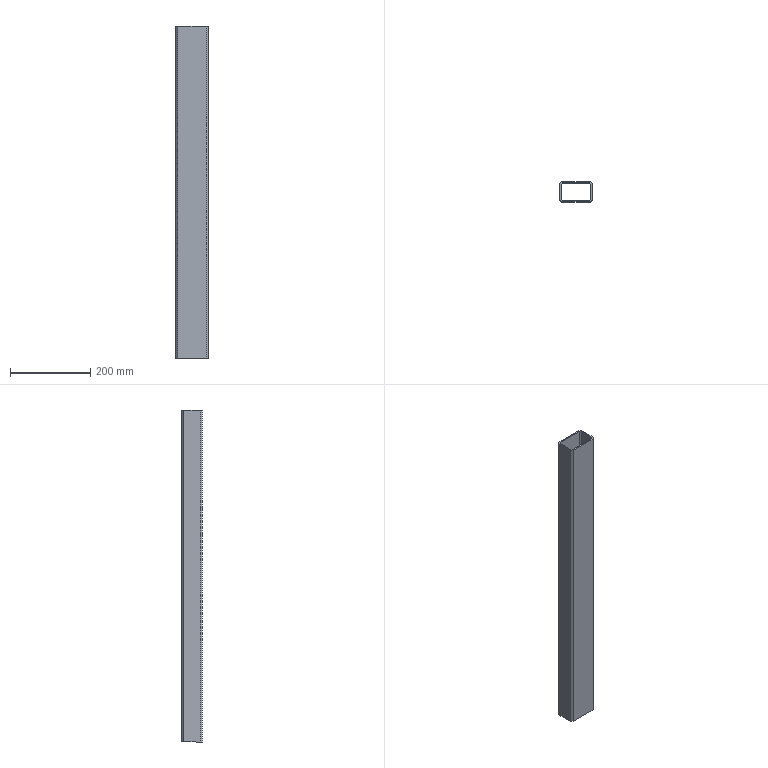Part | SolidWorks | features BaseBody 1 | 1 solid | 18 faces | box 80 x 50 x 825 mm | volume 589899 mm3 | plane 18
STEP:
#1=CARTESIAN_POINT('',(43.047,1567.079,-399.));
#2=VERTEX_POINT('',#1);
#3=CARTESIAN_POINT('',(113.047,1567.079,-399.));
#4=VERTEX_POINT('',#3);
#5=CARTESIAN_POINT('',(38.047,1567.079,-399.));
#6=DIRECTION('',(1.,0.,0.));
#7=VECTOR('',#6,1000.);
#8=LINE('',#5,#7);
#9=EDGE_CURVE('',#2,#4,#8,.T.);
#10=ORIENTED_EDGE('',*,*,#9,.F.);
#11=CARTESIAN_POINT('',(43.047,1567.079,-1224.));
#12=VERTEX_POINT('',#11);
#13=CARTESIAN_POINT('',(43.047,1567.079,-449.));
#14=DIRECTION('',(0.,0.,1.));
#15=VECTOR('',#14,1000.);
#16=LINE('',#13,#15);
#17=EDGE_CURVE('',#12,#2,#16,.T.);
#18=ORIENTED_EDGE('',*,*,#17,.F.);
#19=CARTESIAN_POINT('',(113.047,1567.079,-1224.));
#20=VERTEX_POINT('',#19);
#21=CARTESIAN_POINT('',(38.047,1567.079,-1224.));
#22=DIRECTION('',(-1.,0.,0.));
#23=VECTOR('',#22,1000.);
#24=LINE('',#21,#23);
#25=EDGE_CURVE('',#20,#12,#24,.T.);
#26=ORIENTED_EDGE('',*,*,#25,.F.);
#27=CARTESIAN_POINT('',(113.047,1567.079,-449.));
#28=DIRECTION('',(0.,0.,-1.));
#29=VECTOR('',#28,1000.);
#30=LINE('',#27,#29);
#31=EDGE_CURVE('',#4,#20,#30,.T.);
#32=ORIENTED_EDGE('',*,*,#31,.F.);
#33=EDGE_LOOP('',(#10,#18,#26,#32));
#34=FACE_OUTER_BOUND('',#33,.T.);
#35=CARTESIAN_POINT('',(38.047,1567.079,-449.));
#36=DIRECTION('',(0.,1.,0.));
#37=DIRECTION('',(0.,0.,1.));
#38=AXIS2_PLACEMENT_3D('',#35,#36,#37);
#39=PLANE('',#38);
#40=ADVANCED_FACE('',(#34),#39,.F.);
#41=CARTESIAN_POINT('',(118.047,1572.079,-1224.));
#42=VERTEX_POINT('',#41);
#43=CARTESIAN_POINT('',(118.047,1572.079,-1224.));
#44=DIRECTION('',(-0.7071,-0.7071,0.));
#45=VECTOR('',#44,1000.);
#46=LINE('',#43,#45);
#47=EDGE_CURVE('',#42,#20,#46,.T.);
#48=ORIENTED_EDGE('',*,*,#47,.F.);
#49=CARTESIAN_POINT('',(118.047,1572.079,-399.));
#50=VERTEX_POINT('',#49);
#51=CARTESIAN_POINT('',(118.047,1572.079,-449.));
#52=DIRECTION('',(0.,0.,-1.));
#53=VECTOR('',#52,1000.);
#54=LINE('',#51,#53);
#55=EDGE_CURVE('',#50,#42,#54,.T.);
#56=ORIENTED_EDGE('',*,*,#55,.F.);
#57=CARTESIAN_POINT('',(118.047,1572.079,-399.));
#58=DIRECTION('',(0.7071,0.7071,0.));
#59=VECTOR('',#58,1000.);
#60=LINE('',#57,#59);
#61=EDGE_CURVE('',#4,#50,#60,.T.);
#62=ORIENTED_EDGE('',*,*,#61,.F.);
#63=ORIENTED_EDGE('',*,*,#31,.T.);
#64=EDGE_LOOP('',(#48,#56,#62,#63));
#65=FACE_OUTER_BOUND('',#64,.T.);
#66=CARTESIAN_POINT('',(118.047,1572.079,-449.));
#67=DIRECTION('',(-0.7071,0.7071,0.));
#68=DIRECTION('',(-0.7071,-0.7071,0.));
#69=AXIS2_PLACEMENT_3D('',#66,#67,#68);
#70=PLANE('',#69);
#71=ADVANCED_FACE('',(#65),#70,.F.);
#72=CARTESIAN_POINT('',(115.047,1573.321,-399.));
#73=VERTEX_POINT('',#72);
#74=CARTESIAN_POINT('',(111.804,1570.079,-399.));
#75=VERTEX_POINT('',#74);
#76=CARTESIAN_POINT('',(115.047,1573.321,-399.));
#77=DIRECTION('',(-0.7071,-0.7071,0.));
#78=VECTOR('',#77,1000.);
#79=LINE('',#76,#78);
#80=EDGE_CURVE('',#73,#75,#79,.T.);
#81=ORIENTED_EDGE('',*,*,#80,.T.);
#82=CARTESIAN_POINT('',(44.289,1570.079,-399.));
#83=VERTEX_POINT('',#82);
#84=CARTESIAN_POINT('',(118.047,1570.079,-399.));
#85=DIRECTION('',(-1.,0.,0.));
#86=VECTOR('',#85,1000.);
#87=LINE('',#84,#86);
#88=EDGE_CURVE('',#75,#83,#87,.T.);
#89=ORIENTED_EDGE('',*,*,#88,.T.);
#90=CARTESIAN_POINT('',(41.047,1573.321,-399.));
#91=VERTEX_POINT('',#90);
#92=CARTESIAN_POINT('',(44.289,1570.079,-399.));
#93=DIRECTION('',(-0.7071,0.7071,0.));
#94=VECTOR('',#93,1000.);
#95=LINE('',#92,#94);
#96=EDGE_CURVE('',#83,#91,#95,.T.);
#97=ORIENTED_EDGE('',*,*,#96,.T.);
#98=CARTESIAN_POINT('',(41.047,1610.836,-399.));
#99=VERTEX_POINT('',#98);
#100=CARTESIAN_POINT('',(41.047,1567.079,-399.));
#101=DIRECTION('',(0.,1.,0.));
#102=VECTOR('',#101,1000.);
#103=LINE('',#100,#102);
#104=EDGE_CURVE('',#91,#99,#103,.T.);
#105=ORIENTED_EDGE('',*,*,#104,.T.);
#106=CARTESIAN_POINT('',(44.289,1614.079,-399.));
#107=VERTEX_POINT('',#106);
#108=CARTESIAN_POINT('',(41.047,1610.836,-399.));
#109=DIRECTION('',(0.7071,0.7071,0.));
#110=VECTOR('',#109,1000.);
#111=LINE('',#108,#110);
#112=EDGE_CURVE('',#99,#107,#111,.T.);
#113=ORIENTED_EDGE('',*,*,#112,.T.);
#114=CARTESIAN_POINT('',(111.804,1614.079,-399.));
#115=VERTEX_POINT('',#114);
#116=CARTESIAN_POINT('',(118.047,1614.079,-399.));
#117=DIRECTION('',(1.,0.,0.));
#118=VECTOR('',#117,1000.);
#119=LINE('',#116,#118);
#120=EDGE_CURVE('',#107,#115,#119,.T.);
#121=ORIENTED_EDGE('',*,*,#120,.T.);
#122=CARTESIAN_POINT('',(115.047,1610.836,-399.));
#123=VERTEX_POINT('',#122);
#124=CARTESIAN_POINT('',(111.804,1614.079,-399.));
#125=DIRECTION('',(0.7071,-0.7071,0.));
#126=VECTOR('',#125,1000.);
#127=LINE('',#124,#126);
#128=EDGE_CURVE('',#115,#123,#127,.T.);
#129=ORIENTED_EDGE('',*,*,#128,.T.);
#130=CARTESIAN_POINT('',(115.047,1567.079,-399.));
#131=DIRECTION('',(0.,-1.,0.));
#132=VECTOR('',#131,1000.);
#133=LINE('',#130,#132);
#134=EDGE_CURVE('',#123,#73,#133,.T.);
#135=ORIENTED_EDGE('',*,*,#134,.T.);
#136=EDGE_LOOP('',(#81,#89,#97,#105,#113,#121,#129,#135));
#137=FACE_BOUND('',#136,.T.);
#138=CARTESIAN_POINT('',(38.047,1572.079,-399.));
#139=VERTEX_POINT('',#138);
#140=CARTESIAN_POINT('',(38.047,1572.079,-399.));
#141=DIRECTION('',(0.7071,-0.7071,0.));
#142=VECTOR('',#141,1000.);
#143=LINE('',#140,#142);
#144=EDGE_CURVE('',#139,#2,#143,.T.);
#145=ORIENTED_EDGE('',*,*,#144,.T.);
#146=ORIENTED_EDGE('',*,*,#9,.T.);
#147=ORIENTED_EDGE('',*,*,#61,.T.);
#148=CARTESIAN_POINT('',(118.047,1612.079,-399.));
#149=VERTEX_POINT('',#148);
#150=CARTESIAN_POINT('',(118.047,1567.079,-399.));
#151=DIRECTION('',(0.,1.,0.));
#152=VECTOR('',#151,1000.);
#153=LINE('',#150,#152);
#154=EDGE_CURVE('',#50,#149,#153,.T.);
#155=ORIENTED_EDGE('',*,*,#154,.T.);
#156=CARTESIAN_POINT('',(113.047,1617.079,-399.));
#157=VERTEX_POINT('',#156);
#158=CARTESIAN_POINT('',(118.047,1612.079,-399.));
#159=DIRECTION('',(-0.7071,0.7071,0.));
#160=VECTOR('',#159,1000.);
#161=LINE('',#158,#160);
#162=EDGE_CURVE('',#149,#157,#161,.T.);
#163=ORIENTED_EDGE('',*,*,#162,.T.);
#164=CARTESIAN_POINT('',(43.047,1617.079,-399.));
#165=VERTEX_POINT('',#164);
#166=CARTESIAN_POINT('',(118.047,1617.079,-399.));
#167=DIRECTION('',(-1.,0.,0.));
#168=VECTOR('',#167,1000.);
#169=LINE('',#166,#168);
#170=EDGE_CURVE('',#157,#165,#169,.T.);
#171=ORIENTED_EDGE('',*,*,#170,.T.);
#172=CARTESIAN_POINT('',(38.047,1612.079,-399.));
#173=VERTEX_POINT('',#172);
#174=CARTESIAN_POINT('',(43.047,1617.079,-399.));
#175=DIRECTION('',(-0.7071,-0.7071,0.));
#176=VECTOR('',#175,1000.);
#177=LINE('',#174,#176);
#178=EDGE_CURVE('',#165,#173,#177,.T.);
#179=ORIENTED_EDGE('',*,*,#178,.T.);
#180=CARTESIAN_POINT('',(38.047,1567.079,-399.));
#181=DIRECTION('',(0.,-1.,0.));
#182=VECTOR('',#181,1000.);
#183=LINE('',#180,#182);
#184=EDGE_CURVE('',#173,#139,#183,.T.);
#185=ORIENTED_EDGE('',*,*,#184,.T.);
#186=EDGE_LOOP('',(#145,#146,#147,#155,#163,#171,#179,#185));
#187=FACE_OUTER_BOUND('',#186,.T.);
#188=CARTESIAN_POINT('',(118.047,1567.079,-399.));
#189=DIRECTION('',(0.,0.,1.));
#190=DIRECTION('',(1.,0.,0.));
#191=AXIS2_PLACEMENT_3D('',#188,#189,#190);
#192=PLANE('',#191);
#193=ADVANCED_FACE('',(#137,#187),#192,.T.);
#194=CARTESIAN_POINT('',(38.047,1572.079,-1224.));
#195=VERTEX_POINT('',#194);
#196=CARTESIAN_POINT('',(43.047,1567.079,-1224.));
#197=DIRECTION('',(-0.7071,0.7071,0.));
#198=VECTOR('',#197,1000.);
#199=LINE('',#196,#198);
#200=EDGE_CURVE('',#12,#195,#199,.T.);
#201=ORIENTED_EDGE('',*,*,#200,.F.);
#202=ORIENTED_EDGE('',*,*,#17,.T.);
#203=ORIENTED_EDGE('',*,*,#144,.F.);
#204=CARTESIAN_POINT('',(38.047,1572.079,-449.));
#205=DIRECTION('',(0.,0.,1.));
#206=VECTOR('',#205,1000.);
#207=LINE('',#204,#206);
#208=EDGE_CURVE('',#195,#139,#207,.T.);
#209=ORIENTED_EDGE('',*,*,#208,.F.);
#210=EDGE_LOOP('',(#201,#202,#203,#209));
#211=FACE_OUTER_BOUND('',#210,.T.);
#212=CARTESIAN_POINT('',(43.047,1567.079,-449.));
#213=DIRECTION('',(0.7071,0.7071,0.));
#214=DIRECTION('',(-0.7071,0.7071,0.));
#215=AXIS2_PLACEMENT_3D('',#212,#213,#214);
#216=PLANE('',#215);
#217=ADVANCED_FACE('',(#211),#216,.F.);
#218=CARTESIAN_POINT('',(111.804,1614.079,-1224.));
#219=VERTEX_POINT('',#218);
#220=CARTESIAN_POINT('',(115.047,1610.836,-1224.));
#221=VERTEX_POINT('',#220);
#222=CARTESIAN_POINT('',(111.804,1614.079,-1224.));
#223=DIRECTION('',(0.7071,-0.7071,0.));
#224=VECTOR('',#223,1000.);
#225=LINE('',#222,#224);
#226=EDGE_CURVE('',#219,#221,#225,.T.);
#227=ORIENTED_EDGE('',*,*,#226,.F.);
#228=CARTESIAN_POINT('',(44.289,1614.079,-1224.));
#229=VERTEX_POINT('',#228);
#230=CARTESIAN_POINT('',(118.047,1614.079,-1224.));
#231=DIRECTION('',(1.,0.,0.));
#232=VECTOR('',#231,1000.);
#233=LINE('',#230,#232);
#234=EDGE_CURVE('',#229,#219,#233,.T.);
#235=ORIENTED_EDGE('',*,*,#234,.F.);
#236=CARTESIAN_POINT('',(41.047,1610.836,-1224.));
#237=VERTEX_POINT('',#236);
#238=CARTESIAN_POINT('',(41.047,1610.836,-1224.));
#239=DIRECTION('',(0.7071,0.7071,0.));
#240=VECTOR('',#239,1000.);
#241=LINE('',#238,#240);
#242=EDGE_CURVE('',#237,#229,#241,.T.);
#243=ORIENTED_EDGE('',*,*,#242,.F.);
#244=CARTESIAN_POINT('',(41.047,1573.321,-1224.));
#245=VERTEX_POINT('',#244);
#246=CARTESIAN_POINT('',(41.047,1567.079,-1224.));
#247=DIRECTION('',(0.,1.,0.));
#248=VECTOR('',#247,1000.);
#249=LINE('',#246,#248);
#250=EDGE_CURVE('',#245,#237,#249,.T.);
#251=ORIENTED_EDGE('',*,*,#250,.F.);
#252=CARTESIAN_POINT('',(44.289,1570.079,-1224.));
#253=VERTEX_POINT('',#252);
#254=CARTESIAN_POINT('',(44.289,1570.079,-1224.));
#255=DIRECTION('',(-0.7071,0.7071,0.));
#256=VECTOR('',#255,1000.);
#257=LINE('',#254,#256);
#258=EDGE_CURVE('',#253,#245,#257,.T.);
#259=ORIENTED_EDGE('',*,*,#258,.F.);
#260=CARTESIAN_POINT('',(111.804,1570.079,-1224.));
#261=VERTEX_POINT('',#260);
#262=CARTESIAN_POINT('',(118.047,1570.079,-1224.));
#263=DIRECTION('',(-1.,0.,0.));
#264=VECTOR('',#263,1000.);
#265=LINE('',#262,#264);
#266=EDGE_CURVE('',#261,#253,#265,.T.);
#267=ORIENTED_EDGE('',*,*,#266,.F.);
#268=CARTESIAN_POINT('',(115.047,1573.321,-1224.));
#269=VERTEX_POINT('',#268);
#270=CARTESIAN_POINT('',(115.047,1573.321,-1224.));
#271=DIRECTION('',(-0.7071,-0.7071,0.));
#272=VECTOR('',#271,1000.);
#273=LINE('',#270,#272);
#274=EDGE_CURVE('',#269,#261,#273,.T.);
#275=ORIENTED_EDGE('',*,*,#274,.F.);
#276=CARTESIAN_POINT('',(115.047,1567.079,-1224.));
#277=DIRECTION('',(0.,-1.,0.));
#278=VECTOR('',#277,1000.);
#279=LINE('',#276,#278);
#280=EDGE_CURVE('',#221,#269,#279,.T.);
#281=ORIENTED_EDGE('',*,*,#280,.F.);
#282=EDGE_LOOP('',(#227,#235,#243,#251,#259,#267,#275,#281));
#283=FACE_BOUND('',#282,.T.);
#284=ORIENTED_EDGE('',*,*,#25,.T.);
#285=ORIENTED_EDGE('',*,*,#200,.T.);
#286=CARTESIAN_POINT('',(38.047,1612.079,-1224.));
#287=VERTEX_POINT('',#286);
#288=CARTESIAN_POINT('',(38.047,1567.079,-1224.));
#289=DIRECTION('',(0.,-1.,0.));
#290=VECTOR('',#289,1000.);
#291=LINE('',#288,#290);
#292=EDGE_CURVE('',#287,#195,#291,.T.);
#293=ORIENTED_EDGE('',*,*,#292,.F.);
#294=CARTESIAN_POINT('',(43.047,1617.079,-1224.));
#295=VERTEX_POINT('',#294);
#296=CARTESIAN_POINT('',(43.047,1617.079,-1224.));
#297=DIRECTION('',(-0.7071,-0.7071,0.));
#298=VECTOR('',#297,1000.);
#299=LINE('',#296,#298);
#300=EDGE_CURVE('',#295,#287,#299,.T.);
#301=ORIENTED_EDGE('',*,*,#300,.F.);
#302=CARTESIAN_POINT('',(113.047,1617.079,-1224.));
#303=VERTEX_POINT('',#302);
#304=CARTESIAN_POINT('',(118.047,1617.079,-1224.));
#305=DIRECTION('',(-1.,0.,0.));
#306=VECTOR('',#305,1000.);
#307=LINE('',#304,#306);
#308=EDGE_CURVE('',#303,#295,#307,.T.);
#309=ORIENTED_EDGE('',*,*,#308,.F.);
#310=CARTESIAN_POINT('',(118.047,1612.079,-1224.));
#311=VERTEX_POINT('',#310);
#312=CARTESIAN_POINT('',(118.047,1612.079,-1224.));
#313=DIRECTION('',(-0.7071,0.7071,0.));
#314=VECTOR('',#313,1000.);
#315=LINE('',#312,#314);
#316=EDGE_CURVE('',#311,#303,#315,.T.);
#317=ORIENTED_EDGE('',*,*,#316,.F.);
#318=CARTESIAN_POINT('',(118.047,1567.079,-1224.));
#319=DIRECTION('',(0.,1.,0.));
#320=VECTOR('',#319,1000.);
#321=LINE('',#318,#320);
#322=EDGE_CURVE('',#42,#311,#321,.T.);
#323=ORIENTED_EDGE('',*,*,#322,.F.);
#324=ORIENTED_EDGE('',*,*,#47,.T.);
#325=EDGE_LOOP('',(#284,#285,#293,#301,#309,#317,#323,#324));
#326=FACE_OUTER_BOUND('',#325,.T.);
#327=CARTESIAN_POINT('',(118.047,1567.079,-1224.));
#328=DIRECTION('',(0.,0.,1.));
#329=DIRECTION('',(1.,0.,0.));
#330=AXIS2_PLACEMENT_3D('',#327,#328,#329);
#331=PLANE('',#330);
#332=ADVANCED_FACE('',(#283,#326),#331,.F.);
#333=ORIENTED_EDGE('',*,*,#322,.T.);
#334=CARTESIAN_POINT('',(118.047,1612.079,-449.));
#335=DIRECTION('',(0.,0.,-1.));
#336=VECTOR('',#335,1000.);
#337=LINE('',#334,#336);
#338=EDGE_CURVE('',#149,#311,#337,.T.);
#339=ORIENTED_EDGE('',*,*,#338,.F.);
#340=ORIENTED_EDGE('',*,*,#154,.F.);
#341=ORIENTED_EDGE('',*,*,#55,.T.);
#342=EDGE_LOOP('',(#333,#339,#340,#341));
#343=FACE_OUTER_BOUND('',#342,.T.);
#344=CARTESIAN_POINT('',(118.047,1567.079,-449.));
#345=DIRECTION('',(-1.,0.,0.));
#346=DIRECTION('',(0.,0.,1.));
#347=AXIS2_PLACEMENT_3D('',#344,#345,#346);
#348=PLANE('',#347);
#349=ADVANCED_FACE('',(#343),#348,.F.);
#350=CARTESIAN_POINT('',(111.804,1570.079,-449.));
#351=DIRECTION('',(0.,0.,-1.));
#352=VECTOR('',#351,1000.);
#353=LINE('',#350,#352);
#354=EDGE_CURVE('',#75,#261,#353,.T.);
#355=ORIENTED_EDGE('',*,*,#354,.T.);
#356=ORIENTED_EDGE('',*,*,#266,.T.);
#357=CARTESIAN_POINT('',(44.289,1570.079,-449.));
#358=DIRECTION('',(0.,0.,1.));
#359=VECTOR('',#358,1000.);
#360=LINE('',#357,#359);
#361=EDGE_CURVE('',#253,#83,#360,.T.);
#362=ORIENTED_EDGE('',*,*,#361,.T.);
#363=ORIENTED_EDGE('',*,*,#88,.F.);
#364=EDGE_LOOP('',(#355,#356,#362,#363));
#365=FACE_OUTER_BOUND('',#364,.T.);
#366=CARTESIAN_POINT('',(38.047,1570.079,-449.));
#367=DIRECTION('',(0.,1.,0.));
#368=DIRECTION('',(0.,0.,1.));
#369=AXIS2_PLACEMENT_3D('',#366,#367,#368);
#370=PLANE('',#369);
#371=ADVANCED_FACE('',(#365),#370,.T.);
#372=ORIENTED_EDGE('',*,*,#354,.F.);
#373=ORIENTED_EDGE('',*,*,#80,.F.);
#374=CARTESIAN_POINT('',(115.047,1573.321,-449.));
#375=DIRECTION('',(0.,0.,-1.));
#376=VECTOR('',#375,1000.);
#377=LINE('',#374,#376);
#378=EDGE_CURVE('',#73,#269,#377,.T.);
#379=ORIENTED_EDGE('',*,*,#378,.T.);
#380=ORIENTED_EDGE('',*,*,#274,.T.);
#381=EDGE_LOOP('',(#372,#373,#379,#380));
#382=FACE_OUTER_BOUND('',#381,.T.);
#383=CARTESIAN_POINT('',(115.925,1574.2,-449.));
#384=DIRECTION('',(-0.7071,0.7071,0.));
#385=DIRECTION('',(-0.7071,-0.7071,0.));
#386=AXIS2_PLACEMENT_3D('',#383,#384,#385);
#387=PLANE('',#386);
#388=ADVANCED_FACE('',(#382),#387,.T.);
#389=ORIENTED_EDGE('',*,*,#378,.F.);
#390=ORIENTED_EDGE('',*,*,#134,.F.);
#391=CARTESIAN_POINT('',(115.047,1610.836,-449.));
#392=DIRECTION('',(0.,0.,-1.));
#393=VECTOR('',#392,1000.);
#394=LINE('',#391,#393);
#395=EDGE_CURVE('',#123,#221,#394,.T.);
#396=ORIENTED_EDGE('',*,*,#395,.T.);
#397=ORIENTED_EDGE('',*,*,#280,.T.);
#398=EDGE_LOOP('',(#389,#390,#396,#397));
#399=FACE_OUTER_BOUND('',#398,.T.);
#400=CARTESIAN_POINT('',(115.047,1567.079,-449.));
#401=DIRECTION('',(-1.,0.,0.));
#402=DIRECTION('',(0.,0.,1.));
#403=AXIS2_PLACEMENT_3D('',#400,#401,#402);
#404=PLANE('',#403);
#405=ADVANCED_FACE('',(#399),#404,.T.);
#406=ORIENTED_EDGE('',*,*,#395,.F.);
#407=ORIENTED_EDGE('',*,*,#128,.F.);
#408=CARTESIAN_POINT('',(111.804,1614.079,-449.));
#409=DIRECTION('',(0.,0.,-1.));
#410=VECTOR('',#409,1000.);
#411=LINE('',#408,#410);
#412=EDGE_CURVE('',#115,#219,#411,.T.);
#413=ORIENTED_EDGE('',*,*,#412,.T.);
#414=ORIENTED_EDGE('',*,*,#226,.T.);
#415=EDGE_LOOP('',(#406,#407,#413,#414));
#416=FACE_OUTER_BOUND('',#415,.T.);
#417=CARTESIAN_POINT('',(110.925,1614.957,-449.));
#418=DIRECTION('',(-0.7071,-0.7071,0.));
#419=DIRECTION('',(0.7071,-0.7071,0.));
#420=AXIS2_PLACEMENT_3D('',#417,#418,#419);
#421=PLANE('',#420);
#422=ADVANCED_FACE('',(#416),#421,.T.);
#423=ORIENTED_EDGE('',*,*,#412,.F.);
#424=ORIENTED_EDGE('',*,*,#120,.F.);
#425=CARTESIAN_POINT('',(44.289,1614.079,-449.));
#426=DIRECTION('',(0.,0.,-1.));
#427=VECTOR('',#426,1000.);
#428=LINE('',#425,#427);
#429=EDGE_CURVE('',#107,#229,#428,.T.);
#430=ORIENTED_EDGE('',*,*,#429,.T.);
#431=ORIENTED_EDGE('',*,*,#234,.T.);
#432=EDGE_LOOP('',(#423,#424,#430,#431));
#433=FACE_OUTER_BOUND('',#432,.T.);
#434=CARTESIAN_POINT('',(38.047,1614.079,-449.));
#435=DIRECTION('',(0.,-1.,0.));
#436=DIRECTION('',(0.,0.,-1.));
#437=AXIS2_PLACEMENT_3D('',#434,#435,#436);
#438=PLANE('',#437);
#439=ADVANCED_FACE('',(#433),#438,.T.);
#440=ORIENTED_EDGE('',*,*,#429,.F.);
#441=ORIENTED_EDGE('',*,*,#112,.F.);
#442=CARTESIAN_POINT('',(41.047,1610.836,-449.));
#443=DIRECTION('',(0.,0.,-1.));
#444=VECTOR('',#443,1000.);
#445=LINE('',#442,#444);
#446=EDGE_CURVE('',#99,#237,#445,.T.);
#447=ORIENTED_EDGE('',*,*,#446,.T.);
#448=ORIENTED_EDGE('',*,*,#242,.T.);
#449=EDGE_LOOP('',(#440,#441,#447,#448));
#450=FACE_OUTER_BOUND('',#449,.T.);
#451=CARTESIAN_POINT('',(40.168,1609.957,-449.));
#452=DIRECTION('',(0.7071,-0.7071,0.));
#453=DIRECTION('',(0.7071,0.7071,0.));
#454=AXIS2_PLACEMENT_3D('',#451,#452,#453);
#455=PLANE('',#454);
#456=ADVANCED_FACE('',(#450),#455,.T.);
#457=ORIENTED_EDGE('',*,*,#446,.F.);
#458=ORIENTED_EDGE('',*,*,#104,.F.);
#459=CARTESIAN_POINT('',(41.047,1573.321,-449.));
#460=DIRECTION('',(0.,0.,-1.));
#461=VECTOR('',#460,1000.);
#462=LINE('',#459,#461);
#463=EDGE_CURVE('',#91,#245,#462,.T.);
#464=ORIENTED_EDGE('',*,*,#463,.T.);
#465=ORIENTED_EDGE('',*,*,#250,.T.);
#466=EDGE_LOOP('',(#457,#458,#464,#465));
#467=FACE_OUTER_BOUND('',#466,.T.);
#468=CARTESIAN_POINT('',(41.047,1567.079,-449.));
#469=DIRECTION('',(1.,0.,0.));
#470=DIRECTION('',(0.,0.,-1.));
#471=AXIS2_PLACEMENT_3D('',#468,#469,#470);
#472=PLANE('',#471);
#473=ADVANCED_FACE('',(#467),#472,.T.);
#474=ORIENTED_EDGE('',*,*,#463,.F.);
#475=ORIENTED_EDGE('',*,*,#96,.F.);
#476=ORIENTED_EDGE('',*,*,#361,.F.);
#477=ORIENTED_EDGE('',*,*,#258,.T.);
#478=EDGE_LOOP('',(#474,#475,#476,#477));
#479=FACE_OUTER_BOUND('',#478,.T.);
#480=CARTESIAN_POINT('',(45.168,1569.2,-449.));
#481=DIRECTION('',(0.7071,0.7071,0.));
#482=DIRECTION('',(-0.7071,0.7071,0.));
#483=AXIS2_PLACEMENT_3D('',#480,#481,#482);
#484=PLANE('',#483);
#485=ADVANCED_FACE('',(#479),#484,.T.);
#486=ORIENTED_EDGE('',*,*,#292,.T.);
#487=ORIENTED_EDGE('',*,*,#208,.T.);
#488=ORIENTED_EDGE('',*,*,#184,.F.);
#489=CARTESIAN_POINT('',(38.047,1612.079,-449.));
#490=DIRECTION('',(0.,0.,1.));
#491=VECTOR('',#490,1000.);
#492=LINE('',#489,#491);
#493=EDGE_CURVE('',#287,#173,#492,.T.);
#494=ORIENTED_EDGE('',*,*,#493,.F.);
#495=EDGE_LOOP('',(#486,#487,#488,#494));
#496=FACE_OUTER_BOUND('',#495,.T.);
#497=CARTESIAN_POINT('',(38.047,1567.079,-449.));
#498=DIRECTION('',(1.,0.,0.));
#499=DIRECTION('',(0.,0.,-1.));
#500=AXIS2_PLACEMENT_3D('',#497,#498,#499);
#501=PLANE('',#500);
#502=ADVANCED_FACE('',(#496),#501,.F.);
#503=ORIENTED_EDGE('',*,*,#300,.T.);
#504=ORIENTED_EDGE('',*,*,#493,.T.);
#505=ORIENTED_EDGE('',*,*,#178,.F.);
#506=CARTESIAN_POINT('',(43.047,1617.079,-449.));
#507=DIRECTION('',(0.,0.,1.));
#508=VECTOR('',#507,1000.);
#509=LINE('',#506,#508);
#510=EDGE_CURVE('',#295,#165,#509,.T.);
#511=ORIENTED_EDGE('',*,*,#510,.F.);
#512=EDGE_LOOP('',(#503,#504,#505,#511));
#513=FACE_OUTER_BOUND('',#512,.T.);
#514=CARTESIAN_POINT('',(38.047,1612.079,-449.));
#515=DIRECTION('',(0.7071,-0.7071,0.));
#516=DIRECTION('',(0.7071,0.7071,0.));
#517=AXIS2_PLACEMENT_3D('',#514,#515,#516);
#518=PLANE('',#517);
#519=ADVANCED_FACE('',(#513),#518,.F.);
#520=ORIENTED_EDGE('',*,*,#308,.T.);
#521=ORIENTED_EDGE('',*,*,#510,.T.);
#522=ORIENTED_EDGE('',*,*,#170,.F.);
#523=CARTESIAN_POINT('',(113.047,1617.079,-449.));
#524=DIRECTION('',(0.,0.,1.));
#525=VECTOR('',#524,1000.);
#526=LINE('',#523,#525);
#527=EDGE_CURVE('',#303,#157,#526,.T.);
#528=ORIENTED_EDGE('',*,*,#527,.F.);
#529=EDGE_LOOP('',(#520,#521,#522,#528));
#530=FACE_OUTER_BOUND('',#529,.T.);
#531=CARTESIAN_POINT('',(38.047,1617.079,-449.));
#532=DIRECTION('',(0.,-1.,0.));
#533=DIRECTION('',(0.,0.,-1.));
#534=AXIS2_PLACEMENT_3D('',#531,#532,#533);
#535=PLANE('',#534);
#536=ADVANCED_FACE('',(#530),#535,.F.);
#537=ORIENTED_EDGE('',*,*,#316,.T.);
#538=ORIENTED_EDGE('',*,*,#527,.T.);
#539=ORIENTED_EDGE('',*,*,#162,.F.);
#540=ORIENTED_EDGE('',*,*,#338,.T.);
#541=EDGE_LOOP('',(#537,#538,#539,#540));
#542=FACE_OUTER_BOUND('',#541,.T.);
#543=CARTESIAN_POINT('',(113.047,1617.079,-449.));
#544=DIRECTION('',(-0.7071,-0.7071,0.));
#545=DIRECTION('',(0.7071,-0.7071,0.));
#546=AXIS2_PLACEMENT_3D('',#543,#544,#545);
#547=PLANE('',#546);
#548=ADVANCED_FACE('',(#542),#547,.F.);
#549=CLOSED_SHELL('',(#40,#71,#193,#217,#332,#349,#371,#388,#405,#422,#439,#456,#473,#485,#502,#519,#536,#548));
#550=MANIFOLD_SOLID_BREP('',#549);
#551=CARTESIAN_POINT('',(0.,0.,0.));
#552=DIRECTION('',(0.,0.,1.));
#553=DIRECTION('',(1.,0.,0.));
#554=AXIS2_PLACEMENT_3D('',#551,#552,#553);
#555=(LENGTH_UNIT()NAMED_UNIT(*)SI_UNIT(.MILLI.,.METRE.));
#556=UNCERTAINTY_MEASURE_WITH_UNIT(LENGTH_MEASURE(0.00001),#555,'','');
#557=(NAMED_UNIT(*)PLANE_ANGLE_UNIT()SI_UNIT($,.RADIAN.));
#558=(NAMED_UNIT(*)SI_UNIT($,.STERADIAN.)SOLID_ANGLE_UNIT());
#559=(GEOMETRIC_REPRESENTATION_CONTEXT(3)GLOBAL_UNCERTAINTY_ASSIGNED_CONTEXT((#556))GLOBAL_UNIT_ASSIGNED_CONTEXT((#555,#557,#558))REPRESENTATION_CONTEXT('',''));
#560=ADVANCED_BREP_SHAPE_REPRESENTATION('',(#550,#554),#559);